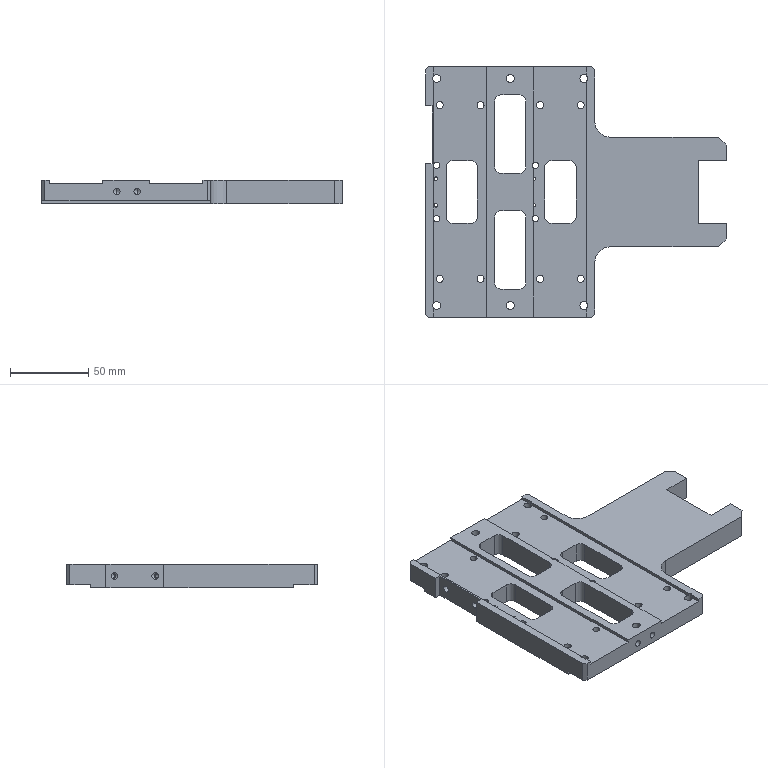Part | NX | features BREP 1 | 1 solid | 200 faces | box 192 x 160 x 15 mm | volume 248558 mm3 | cylinder 102 | plane 66 | cone 32 | commonest cylinder face diameters 8 x32 4.2 x24 4.5 x16 5 x16 4 x8 3.3 x4